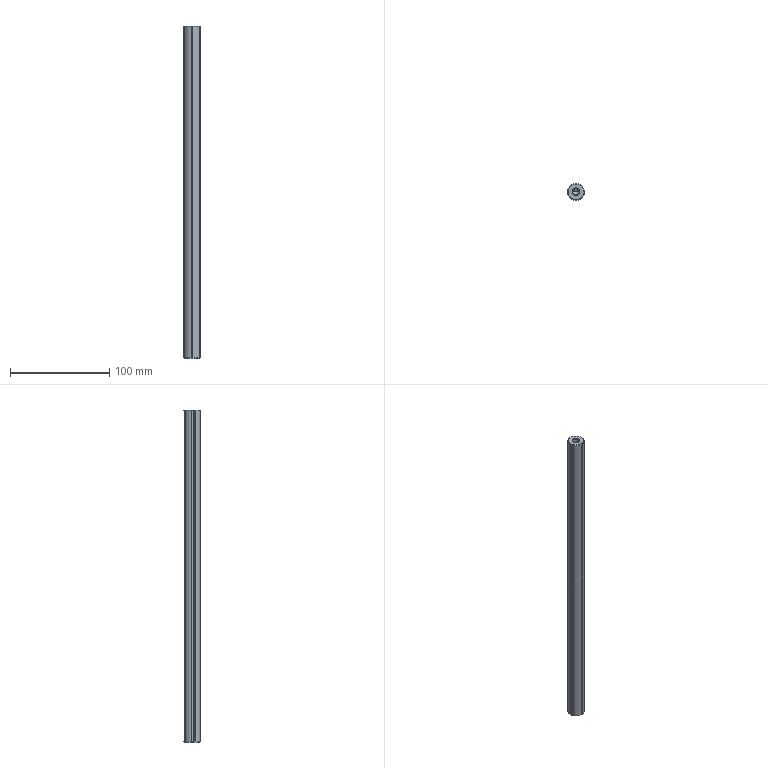Part | STEP file | 0229_Z_BSFM16-335-M8-NTW_1 | 1 solid | 33 faces | box 16.6 x 16.559 x 335 mm | volume 69757 mm3 | cone 16 | cylinder 15 | plane 2 | commonest cylinder face diameters 1.66 x7 16.6 x6 6.647 x2